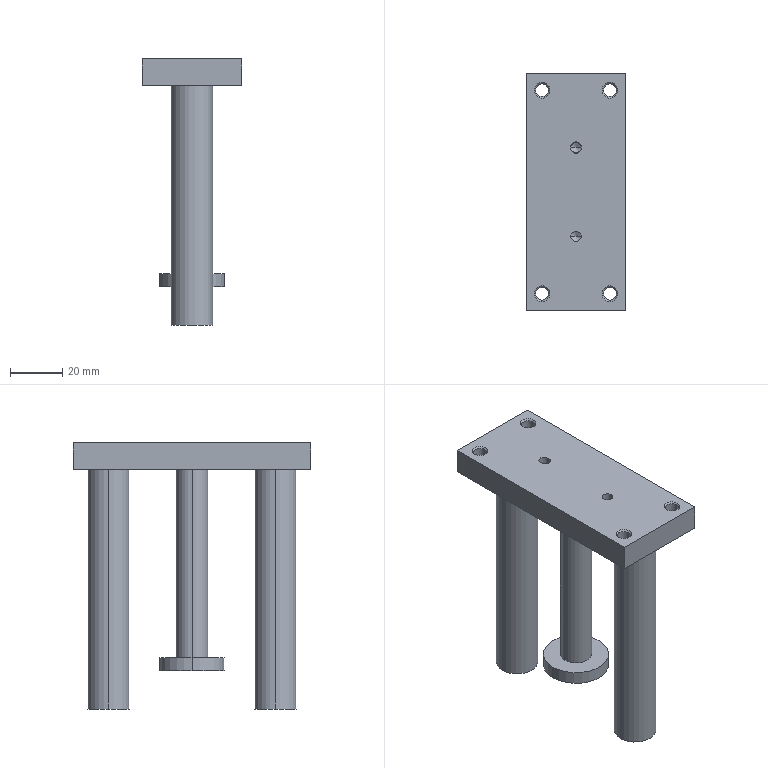Part | SolidWorks | features BaseBody 1 | 1 solid | 56 faces | box 38 x 91 x 102 mm | volume 81256 mm3 | cylinder 22 | cone 20 | plane 14 | commonest cylinder face diameters 4.917 x8 4 x6 16 x4 12 x2 25 x2